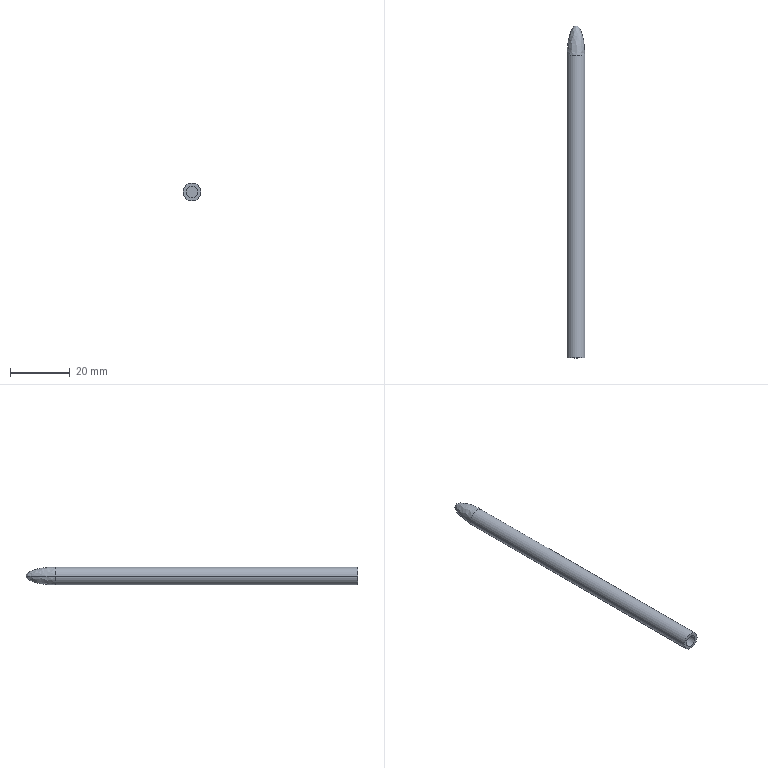Part | SolidWorks | features BaseBody 1 | 1 solid | 8 faces | box 6 x 111 x 6 mm | volume 1788 mm3 | cylinder 4 | plane 2 | spline 2 | commonest cylinder face diameters 4 x2 6 x2
STEP:
#1=CARTESIAN_POINT('',(3.,42.736,0.));
#2=VERTEX_POINT('',#1);
#3=CARTESIAN_POINT('',(-3.,42.736,0.));
#4=VERTEX_POINT('',#3);
#5=CARTESIAN_POINT('',(0.,42.736,0.));
#6=DIRECTION('',(0.,-1.,0.));
#7=DIRECTION('',(1.,0.,0.));
#8=AXIS2_PLACEMENT_3D('',#5,#6,#7);
#9=CIRCLE('',#8,3.);
#10=EDGE_CURVE('',#2,#4,#9,.T.);
#11=ORIENTED_EDGE('',*,*,#10,.T.);
#12=CARTESIAN_POINT('',(-3.,-58.264,0.));
#13=VERTEX_POINT('',#12);
#14=CARTESIAN_POINT('',(-3.,0.,0.));
#15=DIRECTION('',(0.,-1.,0.));
#16=VECTOR('',#15,1000.);
#17=LINE('',#14,#16);
#18=EDGE_CURVE('',#4,#13,#17,.T.);
#19=ORIENTED_EDGE('',*,*,#18,.T.);
#20=CARTESIAN_POINT('',(3.,-58.264,0.));
#21=VERTEX_POINT('',#20);
#22=CARTESIAN_POINT('',(0.,-58.264,0.));
#23=DIRECTION('',(0.,1.,0.));
#24=DIRECTION('',(1.,0.,0.));
#25=AXIS2_PLACEMENT_3D('',#22,#23,#24);
#26=CIRCLE('',#25,3.);
#27=EDGE_CURVE('',#13,#21,#26,.T.);
#28=ORIENTED_EDGE('',*,*,#27,.T.);
#29=CARTESIAN_POINT('',(3.,0.,0.));
#30=DIRECTION('',(0.,-1.,0.));
#31=VECTOR('',#30,1000.);
#32=LINE('',#29,#31);
#33=EDGE_CURVE('',#2,#21,#32,.T.);
#34=ORIENTED_EDGE('',*,*,#33,.F.);
#35=EDGE_LOOP('',(#11,#19,#28,#34));
#36=FACE_OUTER_BOUND('',#35,.T.);
#37=CARTESIAN_POINT('',(0.,0.,0.));
#38=DIRECTION('',(0.,-1.,0.));
#39=DIRECTION('',(1.,0.,0.));
#40=AXIS2_PLACEMENT_3D('',#37,#38,#39);
#41=CYLINDRICAL_SURFACE('',#40,3.);
#42=ADVANCED_FACE('',(#36),#41,.T.);
#43=CARTESIAN_POINT('',(-2.,41.736,0.));
#44=VERTEX_POINT('',#43);
#45=CARTESIAN_POINT('',(2.,41.736,0.));
#46=VERTEX_POINT('',#45);
#47=CARTESIAN_POINT('',(0.,41.736,0.));
#48=DIRECTION('',(0.,-1.,0.));
#49=DIRECTION('',(1.,0.,0.));
#50=AXIS2_PLACEMENT_3D('',#47,#48,#49);
#51=CIRCLE('',#50,2.);
#52=EDGE_CURVE('',#44,#46,#51,.T.);
#53=ORIENTED_EDGE('',*,*,#52,.F.);
#54=CARTESIAN_POINT('',(-2.,-58.264,0.));
#55=VERTEX_POINT('',#54);
#56=CARTESIAN_POINT('',(-2.,0.,0.));
#57=DIRECTION('',(0.,-1.,0.));
#58=VECTOR('',#57,1000.);
#59=LINE('',#56,#58);
#60=EDGE_CURVE('',#44,#55,#59,.T.);
#61=ORIENTED_EDGE('',*,*,#60,.T.);
#62=CARTESIAN_POINT('',(2.,-58.264,0.));
#63=VERTEX_POINT('',#62);
#64=CARTESIAN_POINT('',(0.,-58.264,0.));
#65=DIRECTION('',(0.,-1.,0.));
#66=DIRECTION('',(1.,0.,0.));
#67=AXIS2_PLACEMENT_3D('',#64,#65,#66);
#68=CIRCLE('',#67,2.);
#69=EDGE_CURVE('',#55,#63,#68,.T.);
#70=ORIENTED_EDGE('',*,*,#69,.T.);
#71=CARTESIAN_POINT('',(2.,0.,0.));
#72=DIRECTION('',(0.,-1.,0.));
#73=VECTOR('',#72,1000.);
#74=LINE('',#71,#73);
#75=EDGE_CURVE('',#46,#63,#74,.T.);
#76=ORIENTED_EDGE('',*,*,#75,.F.);
#77=EDGE_LOOP('',(#53,#61,#70,#76));
#78=FACE_OUTER_BOUND('',#77,.T.);
#79=CARTESIAN_POINT('',(0.,0.,0.));
#80=DIRECTION('',(0.,-1.,0.));
#81=DIRECTION('',(1.,0.,0.));
#82=AXIS2_PLACEMENT_3D('',#79,#80,#81);
#83=CYLINDRICAL_SURFACE('',#82,2.);
#84=ADVANCED_FACE('',(#78),#83,.F.);
#85=ORIENTED_EDGE('',*,*,#18,.F.);
#86=CARTESIAN_POINT('',(0.,42.736,0.));
#87=DIRECTION('',(0.,-1.,0.));
#88=DIRECTION('',(1.,0.,0.));
#89=AXIS2_PLACEMENT_3D('',#86,#87,#88);
#90=CIRCLE('',#89,3.);
#91=EDGE_CURVE('',#4,#2,#90,.T.);
#92=ORIENTED_EDGE('',*,*,#91,.T.);
#93=ORIENTED_EDGE('',*,*,#33,.T.);
#94=CARTESIAN_POINT('',(0.,-58.264,0.));
#95=DIRECTION('',(0.,1.,0.));
#96=DIRECTION('',(1.,0.,0.));
#97=AXIS2_PLACEMENT_3D('',#94,#95,#96);
#98=CIRCLE('',#97,3.);
#99=EDGE_CURVE('',#21,#13,#98,.T.);
#100=ORIENTED_EDGE('',*,*,#99,.T.);
#101=EDGE_LOOP('',(#85,#92,#93,#100));
#102=FACE_OUTER_BOUND('',#101,.T.);
#103=CARTESIAN_POINT('',(0.,0.,0.));
#104=DIRECTION('',(0.,-1.,0.));
#105=DIRECTION('',(1.,0.,0.));
#106=AXIS2_PLACEMENT_3D('',#103,#104,#105);
#107=CYLINDRICAL_SURFACE('',#106,3.);
#108=ADVANCED_FACE('',(#102),#107,.T.);
#109=ORIENTED_EDGE('',*,*,#99,.F.);
#110=ORIENTED_EDGE('',*,*,#27,.F.);
#111=EDGE_LOOP('',(#109,#110));
#112=FACE_OUTER_BOUND('',#111,.T.);
#113=CARTESIAN_POINT('',(0.,-58.264,0.));
#114=DIRECTION('',(0.,-1.,0.));
#115=DIRECTION('',(1.,0.,0.));
#116=AXIS2_PLACEMENT_3D('',#113,#114,#115);
#117=CIRCLE('',#116,2.);
#118=EDGE_CURVE('',#63,#55,#117,.T.);
#119=ORIENTED_EDGE('',*,*,#118,.F.);
#120=ORIENTED_EDGE('',*,*,#69,.F.);
#121=EDGE_LOOP('',(#119,#120));
#122=FACE_BOUND('',#121,.T.);
#123=CARTESIAN_POINT('',(-2.,-58.264,0.));
#124=DIRECTION('',(0.,1.,0.));
#125=DIRECTION('',(-1.,0.,0.));
#126=AXIS2_PLACEMENT_3D('',#123,#124,#125);
#127=PLANE('',#126);
#128=ADVANCED_FACE('',(#112,#122),#127,.F.);
#129=CARTESIAN_POINT('',(0.,52.736,0.));
#130=VERTEX_POINT('',#129);
#131=CARTESIAN_POINT('',(0.,52.736,0.));
#132=CARTESIAN_POINT('',(-1.757,52.736,0.));
#133=CARTESIAN_POINT('',(-3.,48.593,0.));
#134=CARTESIAN_POINT('',(-3.,42.736,0.));
#135=(BOUNDED_CURVE()B_SPLINE_CURVE(3,(#131,#132,#133,#134),.UNSPECIFIED.,.F.,.F.)B_SPLINE_CURVE_WITH_KNOTS((4,4),(0.,1.),.UNSPECIFIED.)CURVE()GEOMETRIC_REPRESENTATION_ITEM()RATIONAL_B_SPLINE_CURVE((1.,0.8047,0.8047,1.))REPRESENTATION_ITEM(''));
#136=EDGE_CURVE('',#130,#4,#135,.T.);
#137=ORIENTED_EDGE('',*,*,#136,.T.);
#138=ORIENTED_EDGE('',*,*,#10,.F.);
#139=CARTESIAN_POINT('',(3.,42.736,0.));
#140=CARTESIAN_POINT('',(3.,48.593,0.));
#141=CARTESIAN_POINT('',(1.757,52.736,0.));
#142=CARTESIAN_POINT('',(0.,52.736,0.));
#143=(BOUNDED_CURVE()B_SPLINE_CURVE(3,(#139,#140,#141,#142),.UNSPECIFIED.,.F.,.T.)B_SPLINE_CURVE_WITH_KNOTS((4,4),(0.,1.),.UNSPECIFIED.)CURVE()GEOMETRIC_REPRESENTATION_ITEM()RATIONAL_B_SPLINE_CURVE((1.,0.8047,0.8047,1.))REPRESENTATION_ITEM(''));
#144=EDGE_CURVE('',#2,#130,#143,.T.);
#145=ORIENTED_EDGE('',*,*,#144,.T.);
#146=EDGE_LOOP('',(#137,#138,#145));
#147=FACE_OUTER_BOUND('',#146,.T.);
#148=CARTESIAN_POINT('',(0.,52.736,0.));
#149=CARTESIAN_POINT('',(0.,52.736,0.));
#150=CARTESIAN_POINT('',(0.,52.736,0.));
#151=CARTESIAN_POINT('',(0.,52.736,0.));
#152=CARTESIAN_POINT('',(-1.757,52.736,0.));
#153=CARTESIAN_POINT('',(-1.757,52.736,3.515));
#154=CARTESIAN_POINT('',(1.757,52.736,3.515));
#155=CARTESIAN_POINT('',(1.757,52.736,0.));
#156=CARTESIAN_POINT('',(-3.,48.593,0.));
#157=CARTESIAN_POINT('',(-3.,48.593,6.));
#158=CARTESIAN_POINT('',(3.,48.593,6.));
#159=CARTESIAN_POINT('',(3.,48.593,0.));
#160=CARTESIAN_POINT('',(-3.,42.736,0.));
#161=CARTESIAN_POINT('',(-3.,42.736,6.));
#162=CARTESIAN_POINT('',(3.,42.736,6.));
#163=CARTESIAN_POINT('',(3.,42.736,0.));
#164=(BOUNDED_SURFACE()B_SPLINE_SURFACE(3,3,((#148,#149,#150,#151),(#152,#153,#154,#155),(#156,#157,#158,#159),(#160,#161,#162,#163)),.UNSPECIFIED.,.F.,.F.,.F.)B_SPLINE_SURFACE_WITH_KNOTS((4,4),(4,4),(0.,1.),(0.,1.),.UNSPECIFIED.)GEOMETRIC_REPRESENTATION_ITEM()RATIONAL_B_SPLINE_SURFACE(((1.,0.3333,0.3333,1.),(0.8047,0.2682,0.2682,0.8047),(0.8047,0.2682,0.2682,0.8047),(1.,0.3333,0.3333,1.)))REPRESENTATION_ITEM('')SURFACE());
#165=ADVANCED_FACE('',(#147),#164,.T.);
#166=ORIENTED_EDGE('',*,*,#144,.F.);
#167=ORIENTED_EDGE('',*,*,#91,.F.);
#168=ORIENTED_EDGE('',*,*,#136,.F.);
#169=EDGE_LOOP('',(#166,#167,#168));
#170=FACE_OUTER_BOUND('',#169,.T.);
#171=CARTESIAN_POINT('',(0.,52.736,0.));
#172=CARTESIAN_POINT('',(0.,52.736,0.));
#173=CARTESIAN_POINT('',(0.,52.736,0.));
#174=CARTESIAN_POINT('',(0.,52.736,0.));
#175=CARTESIAN_POINT('',(1.757,52.736,0.));
#176=CARTESIAN_POINT('',(1.757,52.736,-3.515));
#177=CARTESIAN_POINT('',(-1.757,52.736,-3.515));
#178=CARTESIAN_POINT('',(-1.757,52.736,0.));
#179=CARTESIAN_POINT('',(3.,48.593,0.));
#180=CARTESIAN_POINT('',(3.,48.593,-6.));
#181=CARTESIAN_POINT('',(-3.,48.593,-6.));
#182=CARTESIAN_POINT('',(-3.,48.593,0.));
#183=CARTESIAN_POINT('',(3.,42.736,0.));
#184=CARTESIAN_POINT('',(3.,42.736,-6.));
#185=CARTESIAN_POINT('',(-3.,42.736,-6.));
#186=CARTESIAN_POINT('',(-3.,42.736,0.));
#187=(BOUNDED_SURFACE()B_SPLINE_SURFACE(3,3,((#171,#172,#173,#174),(#175,#176,#177,#178),(#179,#180,#181,#182),(#183,#184,#185,#186)),.UNSPECIFIED.,.F.,.F.,.T.)B_SPLINE_SURFACE_WITH_KNOTS((4,4),(4,4),(0.,1.),(0.,1.),.UNSPECIFIED.)GEOMETRIC_REPRESENTATION_ITEM()RATIONAL_B_SPLINE_SURFACE(((1.,0.3333,0.3333,1.),(0.8047,0.2682,0.2682,0.8047),(0.8047,0.2682,0.2682,0.8047),(1.,0.3333,0.3333,1.)))REPRESENTATION_ITEM('')SURFACE());
#188=ADVANCED_FACE('',(#170),#187,.T.);
#189=ORIENTED_EDGE('',*,*,#60,.F.);
#190=CARTESIAN_POINT('',(0.,41.736,0.));
#191=DIRECTION('',(0.,-1.,0.));
#192=DIRECTION('',(1.,0.,0.));
#193=AXIS2_PLACEMENT_3D('',#190,#191,#192);
#194=CIRCLE('',#193,2.);
#195=EDGE_CURVE('',#46,#44,#194,.T.);
#196=ORIENTED_EDGE('',*,*,#195,.F.);
#197=ORIENTED_EDGE('',*,*,#75,.T.);
#198=ORIENTED_EDGE('',*,*,#118,.T.);
#199=EDGE_LOOP('',(#189,#196,#197,#198));
#200=FACE_OUTER_BOUND('',#199,.T.);
#201=CARTESIAN_POINT('',(0.,0.,0.));
#202=DIRECTION('',(0.,-1.,0.));
#203=DIRECTION('',(1.,0.,0.));
#204=AXIS2_PLACEMENT_3D('',#201,#202,#203);
#205=CYLINDRICAL_SURFACE('',#204,2.);
#206=ADVANCED_FACE('',(#200),#205,.F.);
#207=ORIENTED_EDGE('',*,*,#195,.T.);
#208=ORIENTED_EDGE('',*,*,#52,.T.);
#209=EDGE_LOOP('',(#207,#208));
#210=FACE_OUTER_BOUND('',#209,.T.);
#211=CARTESIAN_POINT('',(0.,41.736,0.));
#212=DIRECTION('',(0.,1.,0.));
#213=DIRECTION('',(-1.,0.,0.));
#214=AXIS2_PLACEMENT_3D('',#211,#212,#213);
#215=PLANE('',#214);
#216=ADVANCED_FACE('',(#210),#215,.F.);
#217=CLOSED_SHELL('',(#42,#84,#108,#128,#165,#188,#206,#216));
#218=MANIFOLD_SOLID_BREP('',#217);
#219=CARTESIAN_POINT('',(0.,0.,0.));
#220=DIRECTION('',(0.,0.,1.));
#221=DIRECTION('',(1.,0.,0.));
#222=AXIS2_PLACEMENT_3D('',#219,#220,#221);
#223=(LENGTH_UNIT()NAMED_UNIT(*)SI_UNIT(.MILLI.,.METRE.));
#224=UNCERTAINTY_MEASURE_WITH_UNIT(LENGTH_MEASURE(0.00001),#223,'','');
#225=(NAMED_UNIT(*)PLANE_ANGLE_UNIT()SI_UNIT($,.RADIAN.));
#226=(NAMED_UNIT(*)SI_UNIT($,.STERADIAN.)SOLID_ANGLE_UNIT());
#227=(GEOMETRIC_REPRESENTATION_CONTEXT(3)GLOBAL_UNCERTAINTY_ASSIGNED_CONTEXT((#224))GLOBAL_UNIT_ASSIGNED_CONTEXT((#223,#225,#226))REPRESENTATION_CONTEXT('',''));
#228=ADVANCED_BREP_SHAPE_REPRESENTATION('',(#218,#222),#227);